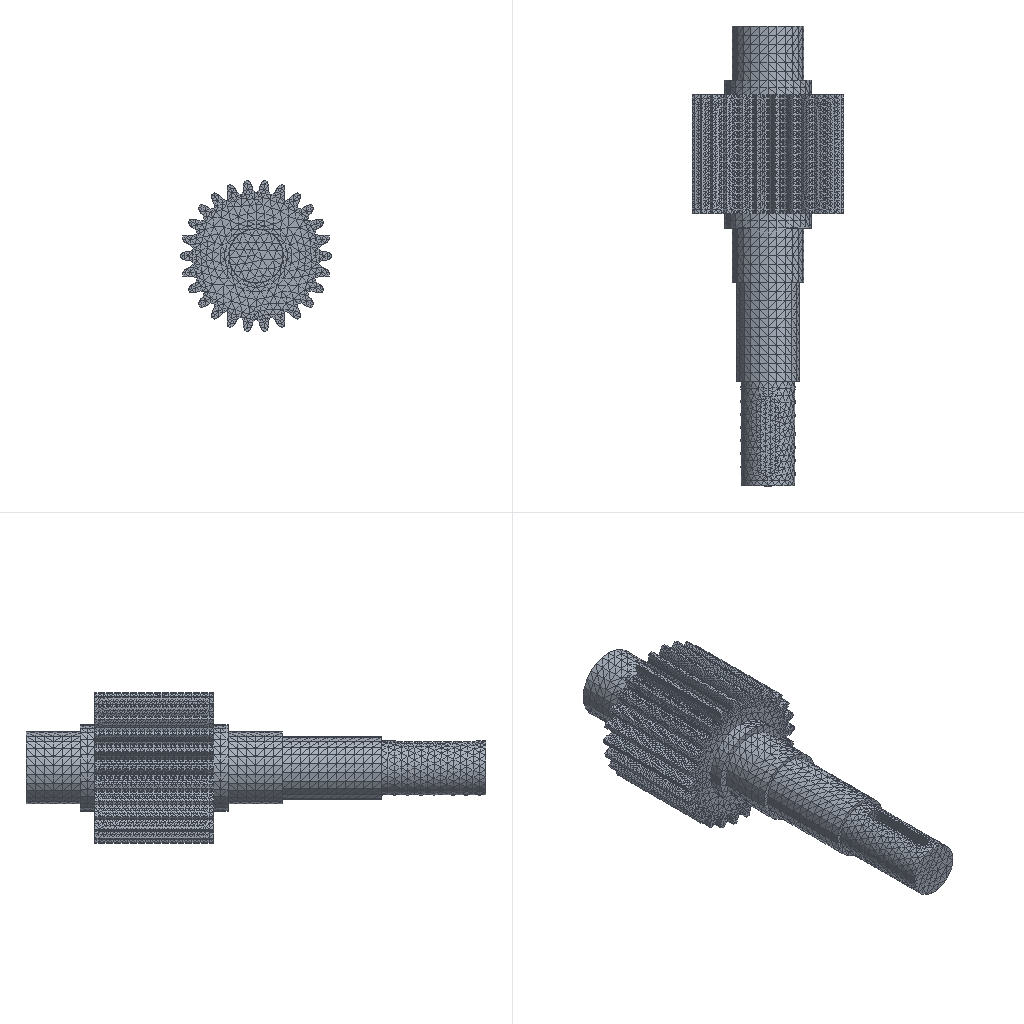Simulation study | nx simcenter
Set-up summary:
category,name,step,type,value,unit,region
solver,nx_nastran (Simcenter)
units,not stated in the deck,,not stated
analysis,deck,,static,static
analysis,solution,,SOL,101
load_step,SUBCASE 1,1,SUBCASE,SPC=1 LOAD=2
load_step,requested,,,1
mesh,nodes,,,102851
mesh,elements,,,63742
element_type,CTETRA,,solid,63742
load,nodal force total,,FX,0.0,model units
load,nodal force total,,FY,0.0,model units
load,nodal force total,,FZ,0.0,model units
load,load commands in deck,,count,2073
bc,support commands in deck,,count,438
analysis,NX solution 0,,Structural,SESTATIC 101 - Single Constraint
check,setup vs results,,match,every grid point's frame and coordinates and every element id; grid points of CTETRA elements
Nastran input file, long lists of numbers shortened:
$*$$$$$$$$$$$$$$$$$$$$$$$$$$$$$$$$$$$$$$$$$$$$$$$$$$$$$$$$$$$$$$$$$
$*
$*                    Simcenter v12.0.0.27 Translator
$*                    for NX Nastran version 12.0
$ (40 more lines like these left out)
ID,NASTRAN,齿轮轴_fem1_sim1-solution_1
SOL 101
CEND
$*
$*$$$$$$$$$$$$$$$$$$$$$$$$$$$$$$$$$$$
$*
$* CASE CONTROL
$*
$*$$$$$$$$$$$$$$$$$$$$$$$$$$$$$$$$$$$
$*
ECHO = NONE
SPC = 1
OUTPUT
DISPLACEMENT(PLOT,REAL) = ALL
SPCFORCES(PLOT,REAL) = ALL
STRESS(PLOT,REAL,VONMISES,CENTER) = ALL
$*  Step: Subcase - Static Loads 1
SUBCASE 1
  LABEL = Subcase - Static Loads 1
  LOAD = 2
$*
$*$$$$$$$$$$$$$$$$$$$$$$$$$$$$$$$$$$$
$*
$* BULK DATA
$*
$*$$$$$$$$$$$$$$$$$$$$$$$$$$$$$$$$$$$
$*
BEGIN BULK
$*
$* PARAM CARDS
$*
PARAM      K6ROT100.0000
PARAM     OIBULK     YES
PARAM    OMACHPR     YES
PARAM       POST      -2
PARAM    POSTEXT     YES
PARAM    UNITSYS   MN-MM
$*
$* GRID CARDS
$*
GRID*                  1               01.8992256777E+002.0044377562E+02+
*       6.3731858137E+00               0
GRID*                  2               05.2213868390E+001.9556098764E+02+
*       6.7960789090E+00               0
$ (205698 more lines like these left out)
$*
$* ELEMENT CARDS
$*
$*  Mesh Collector: Solid(2)
$*  Mesh: 3d_mesh(1)
CTETRA         1       2       1       2       3       4    6420    6421+
+           6422    6423    6424    6425
CTETRA         2       2       1       5       6       4    6426    6427+
+           6428    6423    6429    6430
$ (127480 more lines like these left out)
$*
$* PROPERTY CARDS
$*
$*  Property: PSOLID2
PSOLID         2       1       0                           SMECH
$*
$* MATERIAL CARDS
$*
$*  Material: AISI_410_SS::齿轮轴_fem1::[1]
MAT1           12.1936+8        0.2680007.7338-69.6800-6
MATT1          1       1               2               3
TABLEM1        1                       1                                +
+        20.00002.1936+8 21.11002.1936+8 23.89002.1936+8 37.78002.1867+8+
+        51.67002.1729+8 65.56002.1660+8 79.44002.1591+8 93.33002.1453+8+
+       107.22002.1384+8121.11002.1315+8135.00002.1177+8148.89002.1108+8+
+       162.78002.1039+8176.67002.0901+8190.56002.0832+8204.44002.0694+8+
+       218.33002.0625+8232.22002.0556+8246.11002.0418+8260.00002.0349+8+
+       273.89002.0211+8287.78002.0142+8301.67002.0004+8315.56001.9935+8+
+       329.44001.9866+8343.33001.9728+8357.22001.9659+8371.11001.9521+8+
+       385.00001.9452+8398.89001.9314+8412.78001.9176+8426.67001.9038+8+
+       440.56001.8900+8454.44001.8763+8468.33001.8625+8482.22001.8418+8+
+       496.11001.8280+8510.00001.8073+8523.89001.7866+8537.78001.7659+8+
+       551.67001.7452+8565.56001.7176+8579.44001.6969+8593.33001.6693+8+
+       607.22001.6417+8621.11001.6141+8635.00001.5796+8648.89001.5520+8+
+       662.78001.5176+8676.67001.4831+8690.56001.4417+8704.44001.4072+8+
+           ENDT
TABLEM1        2                       1                                +
+        20.00000.268000 21.11000.268000 23.89000.268000 37.78000.268000+
+        51.67000.268000 65.56000.268000 79.44000.268000 93.33000.268000+
+       107.22000.268000121.11000.268000135.00000.268000148.89000.268000+
+       162.78000.268000176.67000.268000190.56000.268000204.44000.268000+
+       218.33000.268000232.22000.268000246.11000.268000260.00000.268000+
+       273.89000.268000287.78000.268000301.67000.268000315.56000.268000+
+       329.44000.269000343.33000.269000357.22000.269000371.11000.269000+
+       385.00000.270000398.89000.270000412.78000.271000426.67000.271000+
+       440.56000.272000454.44000.273000468.33000.274000482.22000.275000+
+       496.11000.277000510.00000.278000523.89000.280000537.78000.281000+
+       551.67000.283000565.56000.286000579.44000.288000593.33000.290000+
+       607.22000.293000621.11000.295000635.00000.298000648.89000.301000+
+       662.78000.305000676.67000.308000690.56000.311000704.44000.315000+
+           ENDT
TABLEM1        3                       1                                +
+        20.00009.6800-6 93.33001.0080-5107.22001.0152-5121.11001.0224-5+
+       135.00001.0296-5148.89001.0368-5162.78001.0440-5176.67001.0512-5+
+       190.56001.0566-5204.44001.0638-5218.33001.0710-5232.22001.0764-5+
+       246.11001.0836-5260.00001.0890-5273.89001.0944-5287.78001.1016-5+
+       301.67001.1070-5315.56001.1124-5329.44001.1178-5343.33001.1232-5+
+       357.22001.1286-5371.11001.1340-5385.00001.1394-5398.89001.1448-5+
+       412.78001.1484-5426.67001.1538-5440.56001.1574-5454.44001.1610-5+
+       468.33001.1646-5482.22001.1682-5496.11001.1718-5510.00001.1754-5+
+       523.89001.1790-5537.78001.1826-5551.67001.1862-5565.56001.1880-5+
+       579.44001.1916-5593.33001.1952-5607.22001.1988-5621.11001.2006-5+
+       635.00001.2042-5648.89001.2060-5662.78001.2096-5676.67001.2114-5+
+       690.56001.2150-5704.44001.2186-5718.33001.2222-5732.22001.2258-5+
+       746.11001.2294-5760.00001.2348-5773.89001.2384-5787.78001.2438-5+
+       801.67001.2474-5815.56001.2528-5829.44001.2582-5843.33001.2654-5+
+       857.22001.2726-5871.11001.2798-5885.00001.2888-5898.89001.2978-5+
+       912.78001.3068-5926.67001.3158-5940.56001.3266-5954.44001.3374-5+
+       968.33001.3464-5982.22001.3572-5996.11001.3680-5 1010.001.3806-5+
+        1023.891.3914-5 1037.781.4022-5    ENDT
$*
$* LOAD AND CONSTRAINT CARDS
$*
$*  Constraint: Fixed(1)
SPC            1   77132  123456  0.0000
SPC            1   77133  123456  0.0000
SPC            1   77134  123456  0.0000
SPC            1   77135  123456  0.0000
$ (434 more lines like these left out)
$*  Load: Pressure(1)
PLOAD4         2      69 2000.00                           97982   98041
PLOAD4         2     192 2000.00                           77580     319
PLOAD4         2     216 2000.00                           77537     354
PLOAD4         2     221 2000.00                           81801     366
$ (2069 more lines like these left out)
ENDDATA 773d6da6
Results summary:
result,analysis,,,static
result,last_loadstep,,,1
result,primary field,,,displacements
result,max displacement,,,0.001108,model units
result,reaction total,,FX,0.01245,model units
result,reaction total,,FY,1.927,model units
result,reaction total,,FZ,-692439.062,model units
result,NX solution 0,,loadcases,1,mm